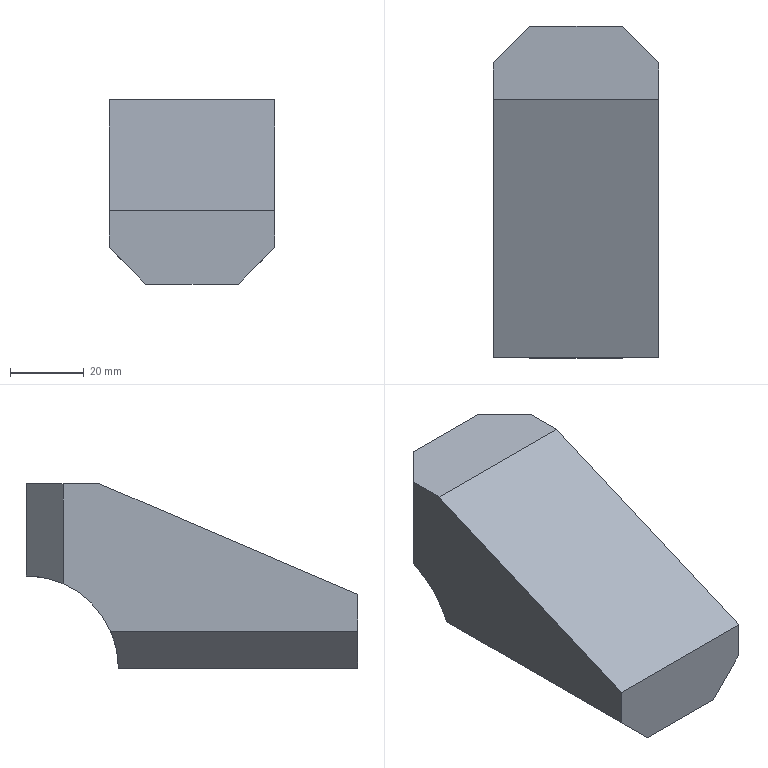Part | SolidWorks | features Chamfer 1, Extrusion 1 | 1 solid | 12 faces | box 45 x 90 x 50 mm | volume 124093 mm3 | plane 11 | cylinder 1 | commonest cylinder face diameters 50 x1
STEP:
#1=CARTESIAN_POINT('',(-22.5,0.,20.));
#2=VERTEX_POINT('',#1);
#3=CARTESIAN_POINT('',(-22.5,0.,10.));
#4=VERTEX_POINT('',#3);
#5=CARTESIAN_POINT('',(-22.5,0.,20.));
#6=DIRECTION('',(0.,0.,-1.));
#7=VECTOR('',#6,1000.);
#8=LINE('',#5,#7);
#9=EDGE_CURVE('',#2,#4,#8,.T.);
#10=ORIENTED_EDGE('',*,*,#9,.T.);
#11=CARTESIAN_POINT('',(-12.5,0.,0.));
#12=VERTEX_POINT('',#11);
#13=CARTESIAN_POINT('',(-12.5,0.,0.));
#14=DIRECTION('',(0.7071,0.,-0.7071));
#15=VECTOR('',#14,1000.);
#16=LINE('',#13,#15);
#17=EDGE_CURVE('',#4,#12,#16,.T.);
#18=ORIENTED_EDGE('',*,*,#17,.T.);
#19=CARTESIAN_POINT('',(12.5,0.,0.));
#20=VERTEX_POINT('',#19);
#21=CARTESIAN_POINT('',(22.5,0.,0.));
#22=DIRECTION('',(-1.,0.,0.));
#23=VECTOR('',#22,1000.);
#24=LINE('',#21,#23);
#25=EDGE_CURVE('',#20,#12,#24,.T.);
#26=ORIENTED_EDGE('',*,*,#25,.F.);
#27=CARTESIAN_POINT('',(22.5,0.,10.));
#28=VERTEX_POINT('',#27);
#29=CARTESIAN_POINT('',(22.5,0.,10.));
#30=DIRECTION('',(0.7071,0.,0.7071));
#31=VECTOR('',#30,1000.);
#32=LINE('',#29,#31);
#33=EDGE_CURVE('',#20,#28,#32,.T.);
#34=ORIENTED_EDGE('',*,*,#33,.T.);
#35=CARTESIAN_POINT('',(22.5,0.,20.));
#36=VERTEX_POINT('',#35);
#37=CARTESIAN_POINT('',(22.5,0.,20.));
#38=DIRECTION('',(0.,0.,-1.));
#39=VECTOR('',#38,1000.);
#40=LINE('',#37,#39);
#41=EDGE_CURVE('',#36,#28,#40,.T.);
#42=ORIENTED_EDGE('',*,*,#41,.F.);
#43=CARTESIAN_POINT('',(22.5,0.,20.));
#44=DIRECTION('',(-1.,0.,0.));
#45=VECTOR('',#44,1000.);
#46=LINE('',#43,#45);
#47=EDGE_CURVE('',#36,#2,#46,.T.);
#48=ORIENTED_EDGE('',*,*,#47,.T.);
#49=EDGE_LOOP('',(#10,#18,#26,#34,#42,#48));
#50=FACE_OUTER_BOUND('',#49,.T.);
#51=CARTESIAN_POINT('',(22.5,0.,20.));
#52=DIRECTION('',(0.,1.,0.));
#53=DIRECTION('',(0.,0.,1.));
#54=AXIS2_PLACEMENT_3D('',#51,#52,#53);
#55=PLANE('',#54);
#56=ADVANCED_FACE('',(#50),#55,.F.);
#57=ORIENTED_EDGE('',*,*,#25,.T.);
#58=CARTESIAN_POINT('',(-12.5,65.,0.));
#59=VERTEX_POINT('',#58);
#60=CARTESIAN_POINT('',(-12.5,0.,0.));
#61=DIRECTION('',(0.,1.,0.));
#62=VECTOR('',#61,1000.);
#63=LINE('',#60,#62);
#64=EDGE_CURVE('',#12,#59,#63,.T.);
#65=ORIENTED_EDGE('',*,*,#64,.T.);
#66=CARTESIAN_POINT('',(12.5,65.,0.));
#67=VERTEX_POINT('',#66);
#68=CARTESIAN_POINT('',(22.5,65.,0.));
#69=DIRECTION('',(-1.,0.,0.));
#70=VECTOR('',#69,1000.);
#71=LINE('',#68,#70);
#72=EDGE_CURVE('',#67,#59,#71,.T.);
#73=ORIENTED_EDGE('',*,*,#72,.F.);
#74=CARTESIAN_POINT('',(12.5,0.,0.));
#75=DIRECTION('',(0.,-1.,0.));
#76=VECTOR('',#75,1000.);
#77=LINE('',#74,#76);
#78=EDGE_CURVE('',#67,#20,#77,.T.);
#79=ORIENTED_EDGE('',*,*,#78,.T.);
#80=EDGE_LOOP('',(#57,#65,#73,#79));
#81=FACE_OUTER_BOUND('',#80,.T.);
#82=CARTESIAN_POINT('',(22.5,0.,0.));
#83=DIRECTION('',(0.,0.,1.));
#84=DIRECTION('',(1.,0.,0.));
#85=AXIS2_PLACEMENT_3D('',#82,#83,#84);
#86=PLANE('',#85);
#87=ADVANCED_FACE('',(#81),#86,.F.);
#88=CARTESIAN_POINT('',(12.5,90.,25.));
#89=VERTEX_POINT('',#88);
#90=CARTESIAN_POINT('',(-12.5,90.,25.));
#91=VERTEX_POINT('',#90);
#92=CARTESIAN_POINT('',(22.5,90.,25.));
#93=DIRECTION('',(-1.,0.,0.));
#94=VECTOR('',#93,1000.);
#95=LINE('',#92,#94);
#96=EDGE_CURVE('',#89,#91,#95,.T.);
#97=ORIENTED_EDGE('',*,*,#96,.F.);
#98=CARTESIAN_POINT('',(22.5,80.,22.913));
#99=VERTEX_POINT('',#98);
#100=CARTESIAN_POINT('',(12.5,90.,25.));
#101=CARTESIAN_POINT('',(15.954,86.546,25.));
#102=CARTESIAN_POINT('',(19.335,83.165,24.294));
#103=CARTESIAN_POINT('',(22.5,80.,22.913));
#104=(BOUNDED_CURVE()B_SPLINE_CURVE(3,(#100,#101,#102,#103),.UNSPECIFIED.,.F.,.F.)B_SPLINE_CURVE_WITH_KNOTS((4,4),(1.571,1.982),.UNSPECIFIED.)CURVE()GEOMETRIC_REPRESENTATION_ITEM()RATIONAL_B_SPLINE_CURVE((1.,0.9859,0.9859,1.))REPRESENTATION_ITEM(''));
#105=EDGE_CURVE('',#89,#99,#104,.T.);
#106=ORIENTED_EDGE('',*,*,#105,.T.);
#107=CARTESIAN_POINT('',(22.5,67.087,10.));
#108=VERTEX_POINT('',#107);
#109=CARTESIAN_POINT('',(22.5,90.,0.));
#110=DIRECTION('',(-1.,0.,0.));
#111=DIRECTION('',(0.,0.,-1.));
#112=AXIS2_PLACEMENT_3D('',#109,#110,#111);
#113=CIRCLE('',#112,25.);
#114=EDGE_CURVE('',#108,#99,#113,.T.);
#115=ORIENTED_EDGE('',*,*,#114,.F.);
#116=CARTESIAN_POINT('',(22.5,67.087,10.));
#117=CARTESIAN_POINT('',(19.335,65.706,6.835));
#118=CARTESIAN_POINT('',(15.954,65.,3.454));
#119=CARTESIAN_POINT('',(12.5,65.,0.));
#120=(BOUNDED_CURVE()B_SPLINE_CURVE(3,(#116,#117,#118,#119),.UNSPECIFIED.,.F.,.F.)B_SPLINE_CURVE_WITH_KNOTS((4,4),(4.301,4.712),.UNSPECIFIED.)CURVE()GEOMETRIC_REPRESENTATION_ITEM()RATIONAL_B_SPLINE_CURVE((1.,0.9859,0.9859,1.))REPRESENTATION_ITEM(''));
#121=EDGE_CURVE('',#108,#67,#120,.T.);
#122=ORIENTED_EDGE('',*,*,#121,.T.);
#123=ORIENTED_EDGE('',*,*,#72,.T.);
#124=CARTESIAN_POINT('',(-22.5,67.087,10.));
#125=VERTEX_POINT('',#124);
#126=CARTESIAN_POINT('',(-12.5,65.,0.));
#127=CARTESIAN_POINT('',(-15.954,65.,3.454));
#128=CARTESIAN_POINT('',(-19.335,65.706,6.835));
#129=CARTESIAN_POINT('',(-22.5,67.087,10.));
#130=(BOUNDED_CURVE()B_SPLINE_CURVE(3,(#126,#127,#128,#129),.UNSPECIFIED.,.F.,.F.)B_SPLINE_CURVE_WITH_KNOTS((4,4),(4.712,5.124),.UNSPECIFIED.)CURVE()GEOMETRIC_REPRESENTATION_ITEM()RATIONAL_B_SPLINE_CURVE((1.,0.9859,0.9859,1.))REPRESENTATION_ITEM(''));
#131=EDGE_CURVE('',#59,#125,#130,.T.);
#132=ORIENTED_EDGE('',*,*,#131,.T.);
#133=CARTESIAN_POINT('',(-22.5,80.,22.913));
#134=VERTEX_POINT('',#133);
#135=CARTESIAN_POINT('',(-22.5,90.,0.));
#136=DIRECTION('',(-1.,0.,0.));
#137=DIRECTION('',(0.,0.,-1.));
#138=AXIS2_PLACEMENT_3D('',#135,#136,#137);
#139=CIRCLE('',#138,25.);
#140=EDGE_CURVE('',#125,#134,#139,.T.);
#141=ORIENTED_EDGE('',*,*,#140,.T.);
#142=CARTESIAN_POINT('',(-22.5,80.,22.913));
#143=CARTESIAN_POINT('',(-19.335,83.165,24.294));
#144=CARTESIAN_POINT('',(-15.954,86.546,25.));
#145=CARTESIAN_POINT('',(-12.5,90.,25.));
#146=(BOUNDED_CURVE()B_SPLINE_CURVE(3,(#142,#143,#144,#145),.UNSPECIFIED.,.F.,.F.)B_SPLINE_CURVE_WITH_KNOTS((4,4),(1.159,1.571),.UNSPECIFIED.)CURVE()GEOMETRIC_REPRESENTATION_ITEM()RATIONAL_B_SPLINE_CURVE((1.,0.9859,0.9859,1.))REPRESENTATION_ITEM(''));
#147=EDGE_CURVE('',#134,#91,#146,.T.);
#148=ORIENTED_EDGE('',*,*,#147,.T.);
#149=EDGE_LOOP('',(#97,#106,#115,#122,#123,#132,#141,#148));
#150=FACE_OUTER_BOUND('',#149,.T.);
#151=CARTESIAN_POINT('',(22.5,90.,0.));
#152=DIRECTION('',(-1.,0.,0.));
#153=DIRECTION('',(0.,0.,1.));
#154=AXIS2_PLACEMENT_3D('',#151,#152,#153);
#155=CYLINDRICAL_SURFACE('',#154,25.);
#156=ADVANCED_FACE('',(#150),#155,.F.);
#157=CARTESIAN_POINT('',(12.5,90.,50.));
#158=VERTEX_POINT('',#157);
#159=CARTESIAN_POINT('',(-12.5,90.,50.));
#160=VERTEX_POINT('',#159);
#161=CARTESIAN_POINT('',(22.5,90.,50.));
#162=DIRECTION('',(-1.,0.,0.));
#163=VECTOR('',#162,1000.);
#164=LINE('',#161,#163);
#165=EDGE_CURVE('',#158,#160,#164,.T.);
#166=ORIENTED_EDGE('',*,*,#165,.F.);
#167=CARTESIAN_POINT('',(12.5,90.,25.));
#168=DIRECTION('',(0.,0.,-1.));
#169=VECTOR('',#168,1000.);
#170=LINE('',#167,#169);
#171=EDGE_CURVE('',#158,#89,#170,.T.);
#172=ORIENTED_EDGE('',*,*,#171,.T.);
#173=ORIENTED_EDGE('',*,*,#96,.T.);
#174=CARTESIAN_POINT('',(-12.5,90.,25.));
#175=DIRECTION('',(0.,0.,1.));
#176=VECTOR('',#175,1000.);
#177=LINE('',#174,#176);
#178=EDGE_CURVE('',#91,#160,#177,.T.);
#179=ORIENTED_EDGE('',*,*,#178,.T.);
#180=EDGE_LOOP('',(#166,#172,#173,#179));
#181=FACE_OUTER_BOUND('',#180,.T.);
#182=CARTESIAN_POINT('',(22.5,90.,25.));
#183=DIRECTION('',(0.,-1.,0.));
#184=DIRECTION('',(0.,0.,-1.));
#185=AXIS2_PLACEMENT_3D('',#182,#183,#184);
#186=PLANE('',#185);
#187=ADVANCED_FACE('',(#181),#186,.F.);
#188=CARTESIAN_POINT('',(22.5,80.,50.));
#189=VERTEX_POINT('',#188);
#190=CARTESIAN_POINT('',(22.5,70.,50.));
#191=VERTEX_POINT('',#190);
#192=CARTESIAN_POINT('',(22.5,90.,50.));
#193=DIRECTION('',(0.,-1.,0.));
#194=VECTOR('',#193,1000.);
#195=LINE('',#192,#194);
#196=EDGE_CURVE('',#189,#191,#195,.T.);
#197=ORIENTED_EDGE('',*,*,#196,.F.);
#198=CARTESIAN_POINT('',(22.5,80.,50.));
#199=DIRECTION('',(-0.7071,0.7071,0.));
#200=VECTOR('',#199,1000.);
#201=LINE('',#198,#200);
#202=EDGE_CURVE('',#189,#158,#201,.T.);
#203=ORIENTED_EDGE('',*,*,#202,.T.);
#204=ORIENTED_EDGE('',*,*,#165,.T.);
#205=CARTESIAN_POINT('',(-22.5,80.,50.));
#206=VERTEX_POINT('',#205);
#207=CARTESIAN_POINT('',(-12.5,90.,50.));
#208=DIRECTION('',(-0.7071,-0.7071,0.));
#209=VECTOR('',#208,1000.);
#210=LINE('',#207,#209);
#211=EDGE_CURVE('',#160,#206,#210,.T.);
#212=ORIENTED_EDGE('',*,*,#211,.T.);
#213=CARTESIAN_POINT('',(-22.5,70.,50.));
#214=VERTEX_POINT('',#213);
#215=CARTESIAN_POINT('',(-22.5,90.,50.));
#216=DIRECTION('',(0.,-1.,0.));
#217=VECTOR('',#216,1000.);
#218=LINE('',#215,#217);
#219=EDGE_CURVE('',#206,#214,#218,.T.);
#220=ORIENTED_EDGE('',*,*,#219,.T.);
#221=CARTESIAN_POINT('',(22.5,70.,50.));
#222=DIRECTION('',(-1.,0.,0.));
#223=VECTOR('',#222,1000.);
#224=LINE('',#221,#223);
#225=EDGE_CURVE('',#191,#214,#224,.T.);
#226=ORIENTED_EDGE('',*,*,#225,.F.);
#227=EDGE_LOOP('',(#197,#203,#204,#212,#220,#226));
#228=FACE_OUTER_BOUND('',#227,.T.);
#229=CARTESIAN_POINT('',(22.5,90.,50.));
#230=DIRECTION('',(0.,0.,-1.));
#231=DIRECTION('',(0.,1.,0.));
#232=AXIS2_PLACEMENT_3D('',#229,#230,#231);
#233=PLANE('',#232);
#234=ADVANCED_FACE('',(#228),#233,.F.);
#235=CARTESIAN_POINT('',(-22.5,70.,50.));
#236=DIRECTION('',(0.,-0.9191,-0.3939));
#237=VECTOR('',#236,1000.);
#238=LINE('',#235,#237);
#239=EDGE_CURVE('',#214,#2,#238,.T.);
#240=ORIENTED_EDGE('',*,*,#239,.T.);
#241=ORIENTED_EDGE('',*,*,#47,.F.);
#242=CARTESIAN_POINT('',(22.5,70.,50.));
#243=DIRECTION('',(0.,-0.9191,-0.3939));
#244=VECTOR('',#243,1000.);
#245=LINE('',#242,#244);
#246=EDGE_CURVE('',#191,#36,#245,.T.);
#247=ORIENTED_EDGE('',*,*,#246,.F.);
#248=ORIENTED_EDGE('',*,*,#225,.T.);
#249=EDGE_LOOP('',(#240,#241,#247,#248));
#250=FACE_OUTER_BOUND('',#249,.T.);
#251=CARTESIAN_POINT('',(22.5,70.,50.));
#252=DIRECTION('',(0.,0.3939,-0.9191));
#253=DIRECTION('',(0.,0.9191,0.3939));
#254=AXIS2_PLACEMENT_3D('',#251,#252,#253);
#255=PLANE('',#254);
#256=ADVANCED_FACE('',(#250),#255,.F.);
#257=ORIENTED_EDGE('',*,*,#114,.T.);
#258=CARTESIAN_POINT('',(22.5,80.,50.));
#259=DIRECTION('',(0.,0.,1.));
#260=VECTOR('',#259,1000.);
#261=LINE('',#258,#260);
#262=EDGE_CURVE('',#99,#189,#261,.T.);
#263=ORIENTED_EDGE('',*,*,#262,.T.);
#264=ORIENTED_EDGE('',*,*,#196,.T.);
#265=ORIENTED_EDGE('',*,*,#246,.T.);
#266=ORIENTED_EDGE('',*,*,#41,.T.);
#267=CARTESIAN_POINT('',(22.5,65.,10.));
#268=DIRECTION('',(0.,1.,0.));
#269=VECTOR('',#268,1000.);
#270=LINE('',#267,#269);
#271=EDGE_CURVE('',#28,#108,#270,.T.);
#272=ORIENTED_EDGE('',*,*,#271,.T.);
#273=EDGE_LOOP('',(#257,#263,#264,#265,#266,#272));
#274=FACE_OUTER_BOUND('',#273,.T.);
#275=CARTESIAN_POINT('',(22.5,90.,0.));
#276=DIRECTION('',(1.,0.,0.));
#277=DIRECTION('',(0.,0.,-1.));
#278=AXIS2_PLACEMENT_3D('',#275,#276,#277);
#279=PLANE('',#278);
#280=ADVANCED_FACE('',(#274),#279,.T.);
#281=ORIENTED_EDGE('',*,*,#219,.F.);
#282=CARTESIAN_POINT('',(-22.5,80.,0.));
#283=DIRECTION('',(0.,0.,-1.));
#284=VECTOR('',#283,1000.);
#285=LINE('',#282,#284);
#286=EDGE_CURVE('',#206,#134,#285,.T.);
#287=ORIENTED_EDGE('',*,*,#286,.T.);
#288=ORIENTED_EDGE('',*,*,#140,.F.);
#289=CARTESIAN_POINT('',(-22.5,90.,10.));
#290=DIRECTION('',(0.,-1.,0.));
#291=VECTOR('',#290,1000.);
#292=LINE('',#289,#291);
#293=EDGE_CURVE('',#125,#4,#292,.T.);
#294=ORIENTED_EDGE('',*,*,#293,.T.);
#295=ORIENTED_EDGE('',*,*,#9,.F.);
#296=ORIENTED_EDGE('',*,*,#239,.F.);
#297=EDGE_LOOP('',(#281,#287,#288,#294,#295,#296));
#298=FACE_OUTER_BOUND('',#297,.T.);
#299=CARTESIAN_POINT('',(-22.5,90.,0.));
#300=DIRECTION('',(1.,0.,0.));
#301=DIRECTION('',(0.,0.,-1.));
#302=AXIS2_PLACEMENT_3D('',#299,#300,#301);
#303=PLANE('',#302);
#304=ADVANCED_FACE('',(#298),#303,.F.);
#305=ORIENTED_EDGE('',*,*,#105,.F.);
#306=ORIENTED_EDGE('',*,*,#171,.F.);
#307=ORIENTED_EDGE('',*,*,#202,.F.);
#308=ORIENTED_EDGE('',*,*,#262,.F.);
#309=EDGE_LOOP('',(#305,#306,#307,#308));
#310=FACE_OUTER_BOUND('',#309,.T.);
#311=CARTESIAN_POINT('',(22.5,80.,0.));
#312=DIRECTION('',(0.7071,0.7071,0.));
#313=DIRECTION('',(0.,0.,-1.));
#314=AXIS2_PLACEMENT_3D('',#311,#312,#313);
#315=PLANE('',#314);
#316=ADVANCED_FACE('',(#310),#315,.T.);
#317=ORIENTED_EDGE('',*,*,#147,.F.);
#318=ORIENTED_EDGE('',*,*,#286,.F.);
#319=ORIENTED_EDGE('',*,*,#211,.F.);
#320=ORIENTED_EDGE('',*,*,#178,.F.);
#321=EDGE_LOOP('',(#317,#318,#319,#320));
#322=FACE_OUTER_BOUND('',#321,.T.);
#323=CARTESIAN_POINT('',(-12.5,90.,25.));
#324=DIRECTION('',(0.7071,-0.7071,0.));
#325=DIRECTION('',(0.,0.,1.));
#326=AXIS2_PLACEMENT_3D('',#323,#324,#325);
#327=PLANE('',#326);
#328=ADVANCED_FACE('',(#322),#327,.F.);
#329=ORIENTED_EDGE('',*,*,#17,.F.);
#330=ORIENTED_EDGE('',*,*,#293,.F.);
#331=ORIENTED_EDGE('',*,*,#131,.F.);
#332=ORIENTED_EDGE('',*,*,#64,.F.);
#333=EDGE_LOOP('',(#329,#330,#331,#332));
#334=FACE_OUTER_BOUND('',#333,.T.);
#335=CARTESIAN_POINT('',(-12.5,0.,0.));
#336=DIRECTION('',(0.7071,0.,0.7071));
#337=DIRECTION('',(0.,1.,0.));
#338=AXIS2_PLACEMENT_3D('',#335,#336,#337);
#339=PLANE('',#338);
#340=ADVANCED_FACE('',(#334),#339,.F.);
#341=ORIENTED_EDGE('',*,*,#33,.F.);
#342=ORIENTED_EDGE('',*,*,#78,.F.);
#343=ORIENTED_EDGE('',*,*,#121,.F.);
#344=ORIENTED_EDGE('',*,*,#271,.F.);
#345=EDGE_LOOP('',(#341,#342,#343,#344));
#346=FACE_OUTER_BOUND('',#345,.T.);
#347=CARTESIAN_POINT('',(22.5,90.,10.));
#348=DIRECTION('',(0.7071,0.,-0.7071));
#349=DIRECTION('',(0.,-1.,0.));
#350=AXIS2_PLACEMENT_3D('',#347,#348,#349);
#351=PLANE('',#350);
#352=ADVANCED_FACE('',(#346),#351,.T.);
#353=CLOSED_SHELL('',(#56,#87,#156,#187,#234,#256,#280,#304,#316,#328,#340,#352));
#354=MANIFOLD_SOLID_BREP('',#353);
#355=CARTESIAN_POINT('',(0.,0.,0.));
#356=DIRECTION('',(0.,0.,1.));
#357=DIRECTION('',(1.,0.,0.));
#358=AXIS2_PLACEMENT_3D('',#355,#356,#357);
#359=(LENGTH_UNIT()NAMED_UNIT(*)SI_UNIT(.MILLI.,.METRE.));
#360=UNCERTAINTY_MEASURE_WITH_UNIT(LENGTH_MEASURE(0.00001),#359,'','');
#361=(NAMED_UNIT(*)PLANE_ANGLE_UNIT()SI_UNIT($,.RADIAN.));
#362=(NAMED_UNIT(*)SI_UNIT($,.STERADIAN.)SOLID_ANGLE_UNIT());
#363=(GEOMETRIC_REPRESENTATION_CONTEXT(3)GLOBAL_UNCERTAINTY_ASSIGNED_CONTEXT((#360))GLOBAL_UNIT_ASSIGNED_CONTEXT((#359,#361,#362))REPRESENTATION_CONTEXT('',''));
#364=ADVANCED_BREP_SHAPE_REPRESENTATION('',(#354,#358),#363);